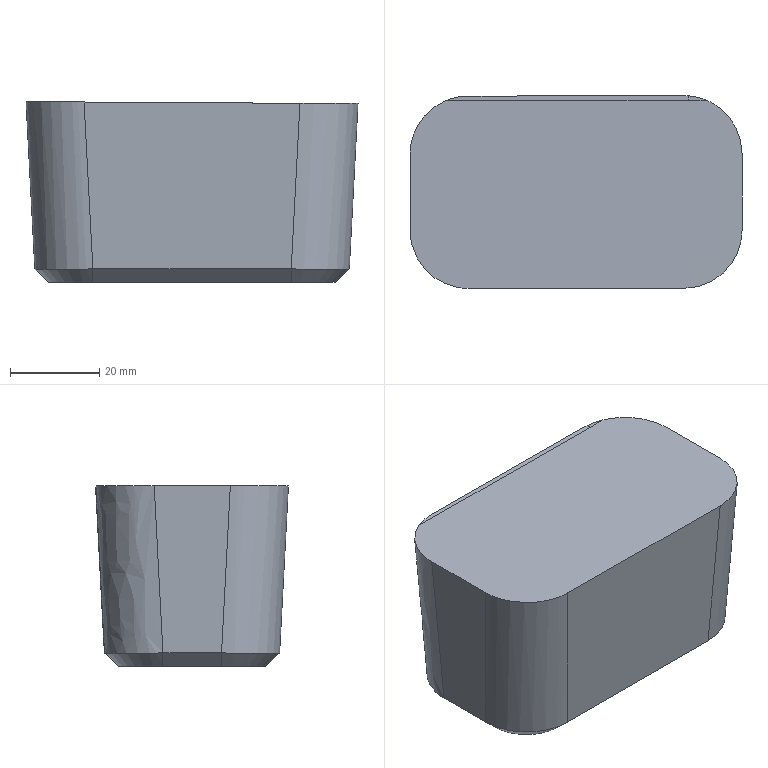Part | STEP file | solid 243 | 1 solid | 25 faces | box 74.214 x 43.098 x 40.392 mm | volume 106427 mm3 | spline 9 | plane 9 | cylinder 4 | cone 2 | other 1 | commonest cylinder face diameters 26 x2 10.2 x1 22 x1